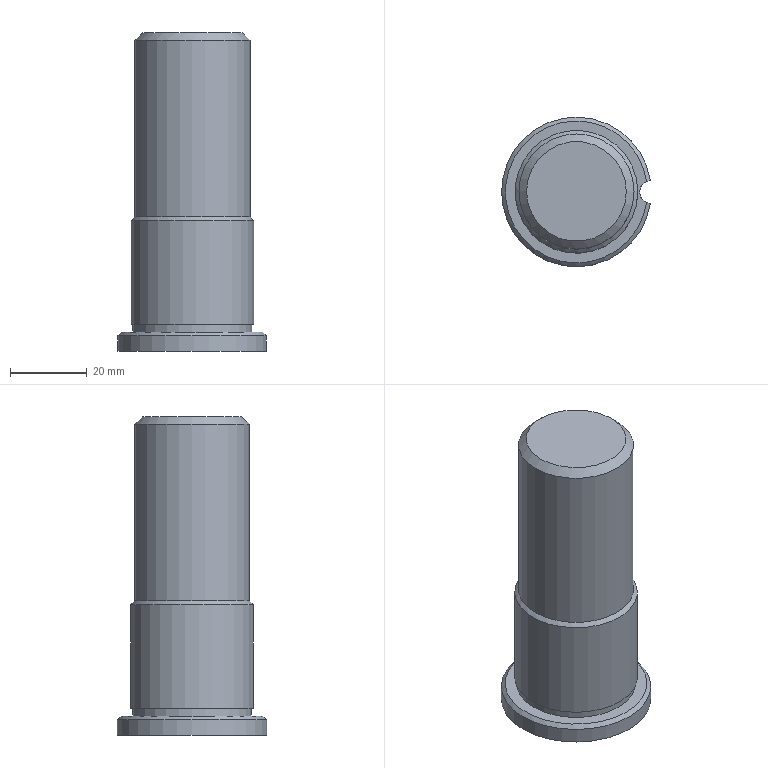Part | NX | features DATUM_CSYS 6, EXTRUDE 5, SKETCH 5, CHAMFER 2 | 1 solid | 12 faces | box 38.769 x 39 x 83 mm | volume 63576 mm3 | cylinder 5 | plane 4 | cone 3 | commonest cylinder face diameters 6 x1 30 x1 31 x1 32 x1 39 x1
STEP:
#1=CARTESIAN_POINT('',(19.269,-2.991,4.));
#2=VERTEX_POINT('',#1);
#3=CARTESIAN_POINT('',(19.269,-2.991,0.));
#4=VERTEX_POINT('',#3);
#5=CARTESIAN_POINT('',(19.269,-2.991,24.));
#6=DIRECTION('',(0.,0.,-1.));
#7=VECTOR('',#6,1000.);
#8=LINE('',#5,#7);
#9=EDGE_CURVE('',#2,#4,#8,.T.);
#10=ORIENTED_EDGE('',*,*,#9,.F.);
#11=CARTESIAN_POINT('',(19.269,2.991,4.));
#12=VERTEX_POINT('',#11);
#13=CARTESIAN_POINT('',(0.,0.,4.));
#14=DIRECTION('',(0.,0.,1.));
#15=DIRECTION('',(1.,0.,0.));
#16=AXIS2_PLACEMENT_3D('',#13,#14,#15);
#17=CIRCLE('',#16,19.5);
#18=EDGE_CURVE('',#2,#12,#17,.F.);
#19=ORIENTED_EDGE('',*,*,#18,.T.);
#20=CARTESIAN_POINT('',(19.269,2.991,0.));
#21=VERTEX_POINT('',#20);
#22=CARTESIAN_POINT('',(19.269,2.991,24.));
#23=DIRECTION('',(0.,0.,-1.));
#24=VECTOR('',#23,1000.);
#25=LINE('',#22,#24);
#26=EDGE_CURVE('',#21,#12,#25,.F.);
#27=ORIENTED_EDGE('',*,*,#26,.F.);
#28=CARTESIAN_POINT('',(0.,0.,0.));
#29=DIRECTION('',(0.,0.,1.));
#30=DIRECTION('',(1.,0.,0.));
#31=AXIS2_PLACEMENT_3D('',#28,#29,#30);
#32=CIRCLE('',#31,19.5);
#33=EDGE_CURVE('',#21,#4,#32,.T.);
#34=ORIENTED_EDGE('',*,*,#33,.T.);
#35=EDGE_LOOP('',(#10,#19,#27,#34));
#36=FACE_BOUND('',#35,.T.);
#37=CARTESIAN_POINT('',(0.,0.,5.));
#38=DIRECTION('',(0.,0.,-1.));
#39=DIRECTION('',(-1.,0.,0.));
#40=AXIS2_PLACEMENT_3D('',#37,#38,#39);
#41=CYLINDRICAL_SURFACE('',#40,19.5);
#42=ADVANCED_FACE('',(#36),#41,.T.);
#43=CARTESIAN_POINT('',(15.5,0.,5.));
#44=VERTEX_POINT('',#43);
#45=CARTESIAN_POINT('',(0.,0.,5.));
#46=DIRECTION('',(0.,0.,1.));
#47=DIRECTION('',(1.,0.,0.));
#48=AXIS2_PLACEMENT_3D('',#45,#46,#47);
#49=CIRCLE('',#48,15.5);
#50=EDGE_CURVE('',#44,#44,#49,.T.);
#51=ORIENTED_EDGE('',*,*,#50,.F.);
#52=EDGE_LOOP('',(#51));
#53=FACE_BOUND('',#52,.T.);
#54=CARTESIAN_POINT('',(18.295,2.747,5.));
#55=VERTEX_POINT('',#54);
#56=CARTESIAN_POINT('',(18.295,-2.747,5.));
#57=VERTEX_POINT('',#56);
#58=CARTESIAN_POINT('',(0.,0.,5.));
#59=DIRECTION('',(0.,0.,1.));
#60=DIRECTION('',(1.,0.,0.));
#61=AXIS2_PLACEMENT_3D('',#58,#59,#60);
#62=CIRCLE('',#61,18.5);
#63=EDGE_CURVE('',#55,#57,#62,.T.);
#64=ORIENTED_EDGE('',*,*,#63,.T.);
#65=CARTESIAN_POINT('',(19.5,0.,5.));
#66=DIRECTION('',(0.,0.,1.));
#67=DIRECTION('',(1.,0.,0.));
#68=AXIS2_PLACEMENT_3D('',#65,#66,#67);
#69=CIRCLE('',#68,3.);
#70=EDGE_CURVE('',#57,#55,#69,.F.);
#71=ORIENTED_EDGE('',*,*,#70,.T.);
#72=EDGE_LOOP('',(#64,#71));
#73=FACE_BOUND('',#72,.T.);
#74=CARTESIAN_POINT('',(0.,0.,5.));
#75=DIRECTION('',(0.,0.,1.));
#76=DIRECTION('',(1.,0.,0.));
#77=AXIS2_PLACEMENT_3D('',#74,#75,#76);
#78=PLANE('',#77);
#79=ADVANCED_FACE('',(#53,#73),#78,.T.);
#80=ORIENTED_EDGE('',*,*,#63,.F.);
#81=CARTESIAN_POINT('',(18.295,2.747,5.));
#82=CARTESIAN_POINT('',(18.608,2.885,4.669));
#83=CARTESIAN_POINT('',(18.933,2.965,4.336));
#84=CARTESIAN_POINT('',(19.269,2.991,4.));
#85=B_SPLINE_CURVE_WITH_KNOTS('',3,(#81,#82,#83,#84),.UNSPECIFIED.,.F.,.F.,(4,4),(0.000000286,0.001418),.UNSPECIFIED.);
#86=EDGE_CURVE('',#55,#12,#85,.T.);
#87=ORIENTED_EDGE('',*,*,#86,.T.);
#88=ORIENTED_EDGE('',*,*,#18,.F.);
#89=CARTESIAN_POINT('',(19.269,-2.991,4.));
#90=CARTESIAN_POINT('',(18.933,-2.965,4.336));
#91=CARTESIAN_POINT('',(18.608,-2.885,4.669));
#92=CARTESIAN_POINT('',(18.295,-2.747,5.));
#93=B_SPLINE_CURVE_WITH_KNOTS('',3,(#89,#90,#91,#92),.UNSPECIFIED.,.F.,.F.,(4,4),(0.000000281,0.001418),.UNSPECIFIED.);
#94=EDGE_CURVE('',#2,#57,#93,.T.);
#95=ORIENTED_EDGE('',*,*,#94,.T.);
#96=EDGE_LOOP('',(#80,#87,#88,#95));
#97=FACE_BOUND('',#96,.T.);
#98=CARTESIAN_POINT('',(0.,0.,5.));
#99=DIRECTION('',(0.,0.,-1.));
#100=DIRECTION('',(-1.,0.,0.));
#101=AXIS2_PLACEMENT_3D('',#98,#99,#100);
#102=CONICAL_SURFACE('',#101,18.5,0.7854);
#103=ADVANCED_FACE('',(#97),#102,.T.);
#104=ORIENTED_EDGE('',*,*,#33,.F.);
#105=CARTESIAN_POINT('',(19.5,0.,0.));
#106=DIRECTION('',(0.,0.,1.));
#107=DIRECTION('',(1.,0.,0.));
#108=AXIS2_PLACEMENT_3D('',#105,#106,#107);
#109=CIRCLE('',#108,3.);
#110=EDGE_CURVE('',#21,#4,#109,.T.);
#111=ORIENTED_EDGE('',*,*,#110,.T.);
#112=EDGE_LOOP('',(#104,#111));
#113=FACE_BOUND('',#112,.T.);
#114=CARTESIAN_POINT('',(0.,0.,0.));
#115=DIRECTION('',(0.,0.,1.));
#116=DIRECTION('',(1.,0.,0.));
#117=AXIS2_PLACEMENT_3D('',#114,#115,#116);
#118=PLANE('',#117);
#119=ADVANCED_FACE('',(#113),#118,.F.);
#120=CARTESIAN_POINT('',(15.5,0.,7.));
#121=VERTEX_POINT('',#120);
#122=CARTESIAN_POINT('',(0.,0.,7.));
#123=DIRECTION('',(0.,0.,1.));
#124=DIRECTION('',(1.,0.,0.));
#125=AXIS2_PLACEMENT_3D('',#122,#123,#124);
#126=CIRCLE('',#125,15.5);
#127=EDGE_CURVE('',#121,#121,#126,.T.);
#128=ORIENTED_EDGE('',*,*,#127,.F.);
#129=EDGE_LOOP('',(#128));
#130=FACE_BOUND('',#129,.T.);
#131=ORIENTED_EDGE('',*,*,#50,.T.);
#132=EDGE_LOOP('',(#131));
#133=FACE_BOUND('',#132,.T.);
#134=CARTESIAN_POINT('',(0.,0.,7.));
#135=DIRECTION('',(0.,0.,-1.));
#136=DIRECTION('',(-1.,0.,0.));
#137=AXIS2_PLACEMENT_3D('',#134,#135,#136);
#138=CYLINDRICAL_SURFACE('',#137,15.5);
#139=ADVANCED_FACE('',(#130,#133),#138,.T.);
#140=CARTESIAN_POINT('',(16.,0.,7.));
#141=VERTEX_POINT('',#140);
#142=CARTESIAN_POINT('',(0.,0.,7.));
#143=DIRECTION('',(0.,0.,1.));
#144=DIRECTION('',(1.,0.,0.));
#145=AXIS2_PLACEMENT_3D('',#142,#143,#144);
#146=CIRCLE('',#145,16.);
#147=EDGE_CURVE('',#141,#141,#146,.T.);
#148=ORIENTED_EDGE('',*,*,#147,.F.);
#149=EDGE_LOOP('',(#148));
#150=FACE_BOUND('',#149,.T.);
#151=ORIENTED_EDGE('',*,*,#127,.T.);
#152=EDGE_LOOP('',(#151));
#153=FACE_BOUND('',#152,.T.);
#154=CARTESIAN_POINT('',(0.,0.,7.));
#155=DIRECTION('',(0.,0.,1.));
#156=DIRECTION('',(1.,0.,0.));
#157=AXIS2_PLACEMENT_3D('',#154,#155,#156);
#158=PLANE('',#157);
#159=ADVANCED_FACE('',(#150,#153),#158,.F.);
#160=CARTESIAN_POINT('',(16.,0.,34.));
#161=VERTEX_POINT('',#160);
#162=CARTESIAN_POINT('',(0.,0.,34.));
#163=DIRECTION('',(0.,0.,1.));
#164=DIRECTION('',(1.,0.,0.));
#165=AXIS2_PLACEMENT_3D('',#162,#163,#164);
#166=CIRCLE('',#165,16.);
#167=EDGE_CURVE('',#161,#161,#166,.F.);
#168=ORIENTED_EDGE('',*,*,#167,.T.);
#169=EDGE_LOOP('',(#168));
#170=FACE_BOUND('',#169,.T.);
#171=ORIENTED_EDGE('',*,*,#147,.T.);
#172=EDGE_LOOP('',(#171));
#173=FACE_BOUND('',#172,.T.);
#174=CARTESIAN_POINT('',(0.,0.,35.));
#175=DIRECTION('',(0.,0.,-1.));
#176=DIRECTION('',(-1.,0.,0.));
#177=AXIS2_PLACEMENT_3D('',#174,#175,#176);
#178=CYLINDRICAL_SURFACE('',#177,16.);
#179=ADVANCED_FACE('',(#170,#173),#178,.T.);
#180=CARTESIAN_POINT('',(15.,0.,81.));
#181=VERTEX_POINT('',#180);
#182=CARTESIAN_POINT('',(0.,0.,81.));
#183=DIRECTION('',(0.,0.,1.));
#184=DIRECTION('',(1.,0.,0.));
#185=AXIS2_PLACEMENT_3D('',#182,#183,#184);
#186=CIRCLE('',#185,15.);
#187=EDGE_CURVE('',#181,#181,#186,.F.);
#188=ORIENTED_EDGE('',*,*,#187,.T.);
#189=EDGE_LOOP('',(#188));
#190=FACE_BOUND('',#189,.T.);
#191=CARTESIAN_POINT('',(15.,0.,35.));
#192=VERTEX_POINT('',#191);
#193=CARTESIAN_POINT('',(0.,0.,35.));
#194=DIRECTION('',(0.,0.,1.));
#195=DIRECTION('',(1.,0.,0.));
#196=AXIS2_PLACEMENT_3D('',#193,#194,#195);
#197=CIRCLE('',#196,15.);
#198=EDGE_CURVE('',#192,#192,#197,.T.);
#199=ORIENTED_EDGE('',*,*,#198,.T.);
#200=EDGE_LOOP('',(#199));
#201=FACE_BOUND('',#200,.T.);
#202=CARTESIAN_POINT('',(0.,0.,83.));
#203=DIRECTION('',(0.,0.,-1.));
#204=DIRECTION('',(-1.,0.,0.));
#205=AXIS2_PLACEMENT_3D('',#202,#203,#204);
#206=CYLINDRICAL_SURFACE('',#205,15.);
#207=ADVANCED_FACE('',(#190,#201),#206,.T.);
#208=CARTESIAN_POINT('',(13.,0.,83.));
#209=VERTEX_POINT('',#208);
#210=CARTESIAN_POINT('',(0.,0.,83.));
#211=DIRECTION('',(0.,0.,1.));
#212=DIRECTION('',(1.,0.,0.));
#213=AXIS2_PLACEMENT_3D('',#210,#211,#212);
#214=CIRCLE('',#213,13.);
#215=EDGE_CURVE('',#209,#209,#214,.T.);
#216=ORIENTED_EDGE('',*,*,#215,.T.);
#217=EDGE_LOOP('',(#216));
#218=FACE_BOUND('',#217,.T.);
#219=CARTESIAN_POINT('',(0.,0.,83.));
#220=DIRECTION('',(0.,0.,1.));
#221=DIRECTION('',(1.,0.,0.));
#222=AXIS2_PLACEMENT_3D('',#219,#220,#221);
#223=PLANE('',#222);
#224=ADVANCED_FACE('',(#218),#223,.T.);
#225=ORIENTED_EDGE('',*,*,#187,.F.);
#226=EDGE_LOOP('',(#225));
#227=FACE_BOUND('',#226,.T.);
#228=ORIENTED_EDGE('',*,*,#215,.F.);
#229=EDGE_LOOP('',(#228));
#230=FACE_BOUND('',#229,.T.);
#231=CARTESIAN_POINT('',(0.,0.,83.));
#232=DIRECTION('',(0.,0.,-1.));
#233=DIRECTION('',(-1.,0.,0.));
#234=AXIS2_PLACEMENT_3D('',#231,#232,#233);
#235=CONICAL_SURFACE('',#234,13.,0.7854);
#236=ADVANCED_FACE('',(#227,#230),#235,.T.);
#237=ORIENTED_EDGE('',*,*,#167,.F.);
#238=EDGE_LOOP('',(#237));
#239=FACE_BOUND('',#238,.T.);
#240=ORIENTED_EDGE('',*,*,#198,.F.);
#241=EDGE_LOOP('',(#240));
#242=FACE_BOUND('',#241,.T.);
#243=CARTESIAN_POINT('',(0.,0.,35.));
#244=DIRECTION('',(0.,0.,-1.));
#245=DIRECTION('',(-1.,0.,0.));
#246=AXIS2_PLACEMENT_3D('',#243,#244,#245);
#247=CONICAL_SURFACE('',#246,15.,0.7854);
#248=ADVANCED_FACE('',(#239,#242),#247,.T.);
#249=ORIENTED_EDGE('',*,*,#26,.T.);
#250=ORIENTED_EDGE('',*,*,#86,.F.);
#251=ORIENTED_EDGE('',*,*,#70,.F.);
#252=ORIENTED_EDGE('',*,*,#94,.F.);
#253=ORIENTED_EDGE('',*,*,#9,.T.);
#254=ORIENTED_EDGE('',*,*,#110,.F.);
#255=EDGE_LOOP('',(#249,#250,#251,#252,#253,#254));
#256=FACE_BOUND('',#255,.T.);
#257=CARTESIAN_POINT('',(19.5,0.,48.));
#258=DIRECTION('',(0.,0.,-1.));
#259=DIRECTION('',(-1.,0.,0.));
#260=AXIS2_PLACEMENT_3D('',#257,#258,#259);
#261=CYLINDRICAL_SURFACE('',#260,3.);
#262=ADVANCED_FACE('',(#256),#261,.F.);
#263=CLOSED_SHELL('',(#42,#79,#103,#119,#139,#159,#179,#207,#224,#236,#248,#262));
#264=MANIFOLD_SOLID_BREP('',#263);
#265=(LENGTH_UNIT()NAMED_UNIT(*)SI_UNIT(.MILLI.,.METRE.));
#266=UNCERTAINTY_MEASURE_WITH_UNIT(LENGTH_MEASURE(0.0508),#265,'','');
#267=(NAMED_UNIT(*)PLANE_ANGLE_UNIT()SI_UNIT($,.RADIAN.));
#268=(NAMED_UNIT(*)SI_UNIT($,.STERADIAN.)SOLID_ANGLE_UNIT());
#269=(GEOMETRIC_REPRESENTATION_CONTEXT(3)GLOBAL_UNCERTAINTY_ASSIGNED_CONTEXT((#266))GLOBAL_UNIT_ASSIGNED_CONTEXT((#265,#267,#268))REPRESENTATION_CONTEXT('',''));
#270=ADVANCED_BREP_SHAPE_REPRESENTATION('',(#264),#269);